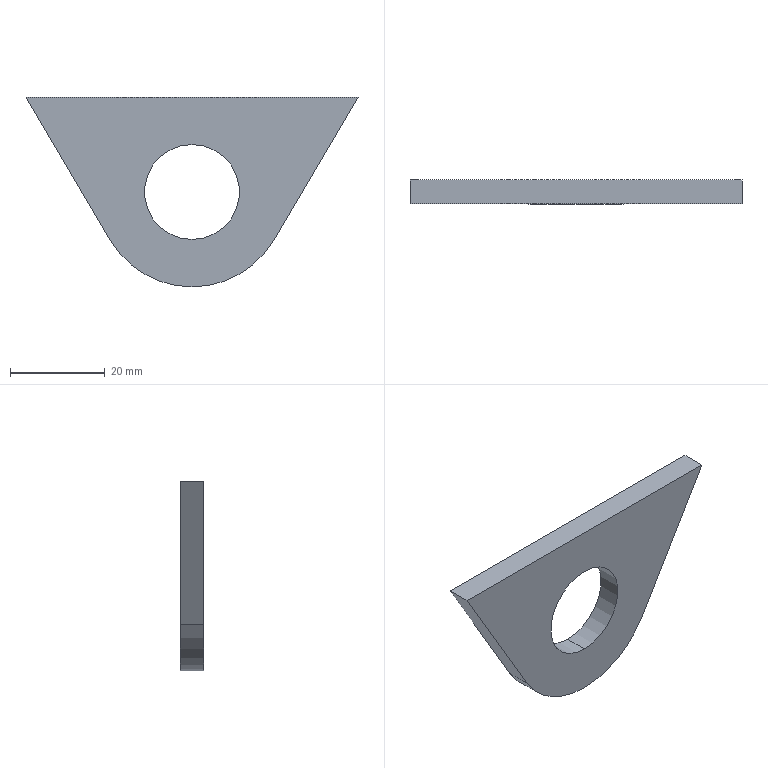Part | SolidWorks | features FlatPattern 1, SMBaseFlange 1, SheetMetal 1 | 1 solid | 9 faces | box 70 x 5 x 40 mm | volume 7506 mm3 | plane 5 | cylinder 4 | commonest cylinder face diameters 20 x2 40 x2
STEP:
#1=CARTESIAN_POINT('',(0.,5.,-10.));
#2=VERTEX_POINT('',#1);
#3=CARTESIAN_POINT('',(0.,5.,10.));
#4=VERTEX_POINT('',#3);
#5=CARTESIAN_POINT('',(0.,5.,0.));
#6=DIRECTION('',(0.,1.,0.));
#7=DIRECTION('',(0.,0.,1.));
#8=AXIS2_PLACEMENT_3D('',#5,#6,#7);
#9=CIRCLE('',#8,10.);
#10=EDGE_CURVE('',#2,#4,#9,.T.);
#11=ORIENTED_EDGE('',*,*,#10,.T.);
#12=CARTESIAN_POINT('',(0.,0.,10.));
#13=VERTEX_POINT('',#12);
#14=CARTESIAN_POINT('',(0.,5.,10.));
#15=DIRECTION('',(0.,-1.,0.));
#16=VECTOR('',#15,1000.);
#17=LINE('',#14,#16);
#18=EDGE_CURVE('',#4,#13,#17,.T.);
#19=ORIENTED_EDGE('',*,*,#18,.T.);
#20=CARTESIAN_POINT('',(0.,0.,-10.));
#21=VERTEX_POINT('',#20);
#22=CARTESIAN_POINT('',(0.,0.,0.));
#23=DIRECTION('',(0.,1.,0.));
#24=DIRECTION('',(0.,0.,1.));
#25=AXIS2_PLACEMENT_3D('',#22,#23,#24);
#26=CIRCLE('',#25,10.);
#27=EDGE_CURVE('',#21,#13,#26,.T.);
#28=ORIENTED_EDGE('',*,*,#27,.F.);
#29=CARTESIAN_POINT('',(0.,5.,-10.));
#30=DIRECTION('',(0.,-1.,0.));
#31=VECTOR('',#30,1000.);
#32=LINE('',#29,#31);
#33=EDGE_CURVE('',#2,#21,#32,.T.);
#34=ORIENTED_EDGE('',*,*,#33,.F.);
#35=EDGE_LOOP('',(#11,#19,#28,#34));
#36=FACE_OUTER_BOUND('',#35,.T.);
#37=CARTESIAN_POINT('',(0.,5.,0.));
#38=DIRECTION('',(0.,-1.,0.));
#39=DIRECTION('',(0.,0.,-1.));
#40=AXIS2_PLACEMENT_3D('',#37,#38,#39);
#41=CYLINDRICAL_SURFACE('',#40,10.);
#42=ADVANCED_FACE('',(#36),#41,.F.);
#43=CARTESIAN_POINT('',(0.,5.,-20.));
#44=VERTEX_POINT('',#43);
#45=CARTESIAN_POINT('',(-17.231,5.,-10.154));
#46=VERTEX_POINT('',#45);
#47=CARTESIAN_POINT('',(0.,5.,0.));
#48=DIRECTION('',(0.,1.,0.));
#49=DIRECTION('',(0.,0.,1.));
#50=AXIS2_PLACEMENT_3D('',#47,#48,#49);
#51=CIRCLE('',#50,20.);
#52=EDGE_CURVE('',#44,#46,#51,.T.);
#53=ORIENTED_EDGE('',*,*,#52,.F.);
#54=CARTESIAN_POINT('',(0.,0.,-20.));
#55=VERTEX_POINT('',#54);
#56=CARTESIAN_POINT('',(0.,5.,-20.));
#57=DIRECTION('',(0.,-1.,0.));
#58=VECTOR('',#57,1000.);
#59=LINE('',#56,#58);
#60=EDGE_CURVE('',#44,#55,#59,.T.);
#61=ORIENTED_EDGE('',*,*,#60,.T.);
#62=CARTESIAN_POINT('',(-17.231,0.,-10.154));
#63=VERTEX_POINT('',#62);
#64=CARTESIAN_POINT('',(0.,0.,0.));
#65=DIRECTION('',(0.,1.,0.));
#66=DIRECTION('',(0.,0.,1.));
#67=AXIS2_PLACEMENT_3D('',#64,#65,#66);
#68=CIRCLE('',#67,20.);
#69=EDGE_CURVE('',#55,#63,#68,.T.);
#70=ORIENTED_EDGE('',*,*,#69,.T.);
#71=CARTESIAN_POINT('',(-17.231,5.,-10.154));
#72=DIRECTION('',(0.,-1.,0.));
#73=VECTOR('',#72,1000.);
#74=LINE('',#71,#73);
#75=EDGE_CURVE('',#46,#63,#74,.T.);
#76=ORIENTED_EDGE('',*,*,#75,.F.);
#77=EDGE_LOOP('',(#53,#61,#70,#76));
#78=FACE_OUTER_BOUND('',#77,.T.);
#79=CARTESIAN_POINT('',(0.,5.,0.));
#80=DIRECTION('',(0.,-1.,0.));
#81=DIRECTION('',(0.,0.,-1.));
#82=AXIS2_PLACEMENT_3D('',#79,#80,#81);
#83=CYLINDRICAL_SURFACE('',#82,20.);
#84=ADVANCED_FACE('',(#78),#83,.T.);
#85=CARTESIAN_POINT('',(35.,5.,20.));
#86=VERTEX_POINT('',#85);
#87=CARTESIAN_POINT('',(17.231,5.,-10.154));
#88=VERTEX_POINT('',#87);
#89=CARTESIAN_POINT('',(35.,5.,20.));
#90=DIRECTION('',(-0.5077,0.,-0.8615));
#91=VECTOR('',#90,1000.);
#92=LINE('',#89,#91);
#93=EDGE_CURVE('',#86,#88,#92,.T.);
#94=ORIENTED_EDGE('',*,*,#93,.T.);
#95=CARTESIAN_POINT('',(0.,5.,0.));
#96=DIRECTION('',(0.,1.,0.));
#97=DIRECTION('',(0.,0.,1.));
#98=AXIS2_PLACEMENT_3D('',#95,#96,#97);
#99=CIRCLE('',#98,20.);
#100=EDGE_CURVE('',#88,#44,#99,.T.);
#101=ORIENTED_EDGE('',*,*,#100,.T.);
#102=ORIENTED_EDGE('',*,*,#52,.T.);
#103=CARTESIAN_POINT('',(-35.,5.,20.));
#104=VERTEX_POINT('',#103);
#105=CARTESIAN_POINT('',(-35.,5.,20.));
#106=DIRECTION('',(-0.5077,0.,0.8615));
#107=VECTOR('',#106,1000.);
#108=LINE('',#105,#107);
#109=EDGE_CURVE('',#46,#104,#108,.T.);
#110=ORIENTED_EDGE('',*,*,#109,.T.);
#111=CARTESIAN_POINT('',(-35.,5.,20.));
#112=DIRECTION('',(1.,0.,0.));
#113=VECTOR('',#112,1000.);
#114=LINE('',#111,#113);
#115=EDGE_CURVE('',#104,#86,#114,.T.);
#116=ORIENTED_EDGE('',*,*,#115,.T.);
#117=EDGE_LOOP('',(#94,#101,#102,#110,#116));
#118=FACE_OUTER_BOUND('',#117,.T.);
#119=ORIENTED_EDGE('',*,*,#10,.F.);
#120=CARTESIAN_POINT('',(0.,5.,0.));
#121=DIRECTION('',(0.,1.,0.));
#122=DIRECTION('',(0.,0.,1.));
#123=AXIS2_PLACEMENT_3D('',#120,#121,#122);
#124=CIRCLE('',#123,10.);
#125=EDGE_CURVE('',#4,#2,#124,.T.);
#126=ORIENTED_EDGE('',*,*,#125,.F.);
#127=EDGE_LOOP('',(#119,#126));
#128=FACE_BOUND('',#127,.T.);
#129=CARTESIAN_POINT('',(0.,5.,0.));
#130=DIRECTION('',(0.,1.,0.));
#131=DIRECTION('',(0.,0.,1.));
#132=AXIS2_PLACEMENT_3D('',#129,#130,#131);
#133=PLANE('',#132);
#134=ADVANCED_FACE('',(#118,#128),#133,.T.);
#135=CARTESIAN_POINT('',(35.,0.,20.));
#136=VERTEX_POINT('',#135);
#137=CARTESIAN_POINT('',(17.231,0.,-10.154));
#138=VERTEX_POINT('',#137);
#139=CARTESIAN_POINT('',(35.,0.,20.));
#140=DIRECTION('',(-0.5077,0.,-0.8615));
#141=VECTOR('',#140,1000.);
#142=LINE('',#139,#141);
#143=EDGE_CURVE('',#136,#138,#142,.T.);
#144=ORIENTED_EDGE('',*,*,#143,.F.);
#145=CARTESIAN_POINT('',(-35.,0.,20.));
#146=VERTEX_POINT('',#145);
#147=CARTESIAN_POINT('',(-35.,0.,20.));
#148=DIRECTION('',(1.,0.,0.));
#149=VECTOR('',#148,1000.);
#150=LINE('',#147,#149);
#151=EDGE_CURVE('',#146,#136,#150,.T.);
#152=ORIENTED_EDGE('',*,*,#151,.F.);
#153=CARTESIAN_POINT('',(-35.,0.,20.));
#154=DIRECTION('',(-0.5077,0.,0.8615));
#155=VECTOR('',#154,1000.);
#156=LINE('',#153,#155);
#157=EDGE_CURVE('',#63,#146,#156,.T.);
#158=ORIENTED_EDGE('',*,*,#157,.F.);
#159=ORIENTED_EDGE('',*,*,#69,.F.);
#160=CARTESIAN_POINT('',(0.,0.,0.));
#161=DIRECTION('',(0.,1.,0.));
#162=DIRECTION('',(0.,0.,1.));
#163=AXIS2_PLACEMENT_3D('',#160,#161,#162);
#164=CIRCLE('',#163,20.);
#165=EDGE_CURVE('',#138,#55,#164,.T.);
#166=ORIENTED_EDGE('',*,*,#165,.F.);
#167=EDGE_LOOP('',(#144,#152,#158,#159,#166));
#168=FACE_OUTER_BOUND('',#167,.T.);
#169=ORIENTED_EDGE('',*,*,#27,.T.);
#170=CARTESIAN_POINT('',(0.,0.,0.));
#171=DIRECTION('',(0.,1.,0.));
#172=DIRECTION('',(0.,0.,1.));
#173=AXIS2_PLACEMENT_3D('',#170,#171,#172);
#174=CIRCLE('',#173,10.);
#175=EDGE_CURVE('',#13,#21,#174,.T.);
#176=ORIENTED_EDGE('',*,*,#175,.T.);
#177=EDGE_LOOP('',(#169,#176));
#178=FACE_BOUND('',#177,.T.);
#179=CARTESIAN_POINT('',(0.,0.,0.));
#180=DIRECTION('',(0.,1.,0.));
#181=DIRECTION('',(0.,0.,1.));
#182=AXIS2_PLACEMENT_3D('',#179,#180,#181);
#183=PLANE('',#182);
#184=ADVANCED_FACE('',(#168,#178),#183,.F.);
#185=ORIENTED_EDGE('',*,*,#143,.T.);
#186=CARTESIAN_POINT('',(17.231,5.,-10.154));
#187=DIRECTION('',(0.,-1.,0.));
#188=VECTOR('',#187,1000.);
#189=LINE('',#186,#188);
#190=EDGE_CURVE('',#88,#138,#189,.T.);
#191=ORIENTED_EDGE('',*,*,#190,.F.);
#192=ORIENTED_EDGE('',*,*,#93,.F.);
#193=CARTESIAN_POINT('',(35.,5.,20.));
#194=DIRECTION('',(0.,-1.,0.));
#195=VECTOR('',#194,1000.);
#196=LINE('',#193,#195);
#197=EDGE_CURVE('',#86,#136,#196,.T.);
#198=ORIENTED_EDGE('',*,*,#197,.T.);
#199=EDGE_LOOP('',(#185,#191,#192,#198));
#200=FACE_OUTER_BOUND('',#199,.T.);
#201=CARTESIAN_POINT('',(35.,5.,20.));
#202=DIRECTION('',(-0.8615,0.,0.5077));
#203=DIRECTION('',(0.5077,0.,0.8615));
#204=AXIS2_PLACEMENT_3D('',#201,#202,#203);
#205=PLANE('',#204);
#206=ADVANCED_FACE('',(#200),#205,.F.);
#207=ORIENTED_EDGE('',*,*,#60,.F.);
#208=ORIENTED_EDGE('',*,*,#100,.F.);
#209=ORIENTED_EDGE('',*,*,#190,.T.);
#210=ORIENTED_EDGE('',*,*,#165,.T.);
#211=EDGE_LOOP('',(#207,#208,#209,#210));
#212=FACE_OUTER_BOUND('',#211,.T.);
#213=CARTESIAN_POINT('',(0.,5.,0.));
#214=DIRECTION('',(0.,-1.,0.));
#215=DIRECTION('',(0.,0.,-1.));
#216=AXIS2_PLACEMENT_3D('',#213,#214,#215);
#217=CYLINDRICAL_SURFACE('',#216,20.);
#218=ADVANCED_FACE('',(#212),#217,.T.);
#219=ORIENTED_EDGE('',*,*,#157,.T.);
#220=CARTESIAN_POINT('',(-35.,5.,20.));
#221=DIRECTION('',(0.,-1.,0.));
#222=VECTOR('',#221,1000.);
#223=LINE('',#220,#222);
#224=EDGE_CURVE('',#104,#146,#223,.T.);
#225=ORIENTED_EDGE('',*,*,#224,.F.);
#226=ORIENTED_EDGE('',*,*,#109,.F.);
#227=ORIENTED_EDGE('',*,*,#75,.T.);
#228=EDGE_LOOP('',(#219,#225,#226,#227));
#229=FACE_OUTER_BOUND('',#228,.T.);
#230=CARTESIAN_POINT('',(-35.,5.,20.));
#231=DIRECTION('',(0.8615,0.,0.5077));
#232=DIRECTION('',(0.5077,0.,-0.8615));
#233=AXIS2_PLACEMENT_3D('',#230,#231,#232);
#234=PLANE('',#233);
#235=ADVANCED_FACE('',(#229),#234,.F.);
#236=ORIENTED_EDGE('',*,*,#151,.T.);
#237=ORIENTED_EDGE('',*,*,#197,.F.);
#238=ORIENTED_EDGE('',*,*,#115,.F.);
#239=ORIENTED_EDGE('',*,*,#224,.T.);
#240=EDGE_LOOP('',(#236,#237,#238,#239));
#241=FACE_OUTER_BOUND('',#240,.T.);
#242=CARTESIAN_POINT('',(-35.,5.,20.));
#243=DIRECTION('',(0.,0.,-1.));
#244=DIRECTION('',(-1.,0.,0.));
#245=AXIS2_PLACEMENT_3D('',#242,#243,#244);
#246=PLANE('',#245);
#247=ADVANCED_FACE('',(#241),#246,.F.);
#248=ORIENTED_EDGE('',*,*,#18,.F.);
#249=ORIENTED_EDGE('',*,*,#125,.T.);
#250=ORIENTED_EDGE('',*,*,#33,.T.);
#251=ORIENTED_EDGE('',*,*,#175,.F.);
#252=EDGE_LOOP('',(#248,#249,#250,#251));
#253=FACE_OUTER_BOUND('',#252,.T.);
#254=CARTESIAN_POINT('',(0.,5.,0.));
#255=DIRECTION('',(0.,-1.,0.));
#256=DIRECTION('',(0.,0.,-1.));
#257=AXIS2_PLACEMENT_3D('',#254,#255,#256);
#258=CYLINDRICAL_SURFACE('',#257,10.);
#259=ADVANCED_FACE('',(#253),#258,.F.);
#260=CLOSED_SHELL('',(#42,#84,#134,#184,#206,#218,#235,#247,#259));
#261=MANIFOLD_SOLID_BREP('',#260);
#262=CARTESIAN_POINT('',(0.,0.,0.));
#263=DIRECTION('',(0.,0.,1.));
#264=DIRECTION('',(1.,0.,0.));
#265=AXIS2_PLACEMENT_3D('',#262,#263,#264);
#266=(LENGTH_UNIT()NAMED_UNIT(*)SI_UNIT(.MILLI.,.METRE.));
#267=UNCERTAINTY_MEASURE_WITH_UNIT(LENGTH_MEASURE(0.00001),#266,'','');
#268=(NAMED_UNIT(*)PLANE_ANGLE_UNIT()SI_UNIT($,.RADIAN.));
#269=(NAMED_UNIT(*)SI_UNIT($,.STERADIAN.)SOLID_ANGLE_UNIT());
#270=(GEOMETRIC_REPRESENTATION_CONTEXT(3)GLOBAL_UNCERTAINTY_ASSIGNED_CONTEXT((#267))GLOBAL_UNIT_ASSIGNED_CONTEXT((#266,#268,#269))REPRESENTATION_CONTEXT('',''));
#271=ADVANCED_BREP_SHAPE_REPRESENTATION('',(#261,#265),#270);